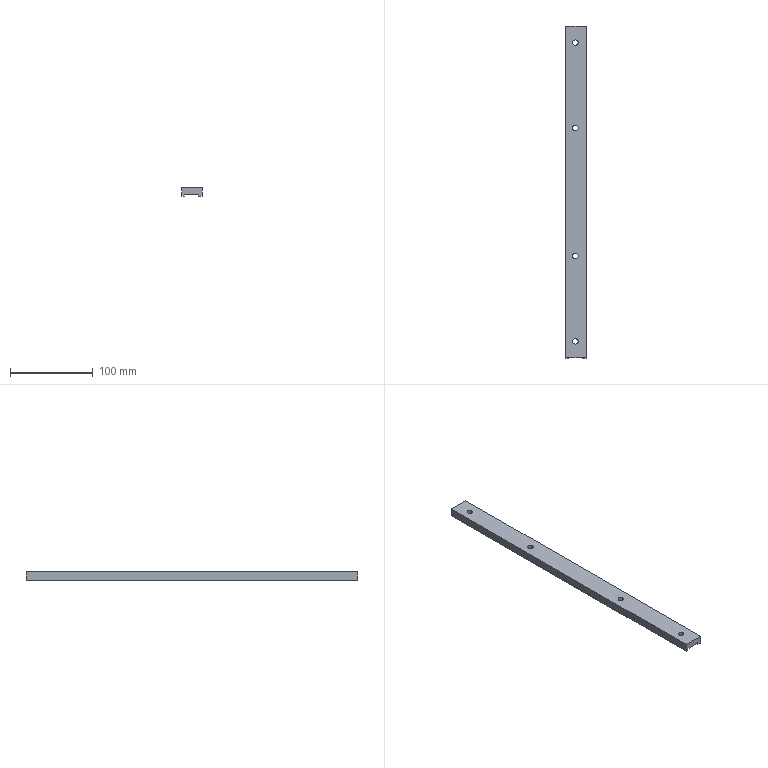Part | SolidWorks | features BaseBody 1 | 1 solid | 26 faces | box 24.5 x 400 x 10 mm | volume 80117 mm3 | plane 10 | cone 8 | cylinder 8 | commonest cylinder face diameters 6.6 x8
STEP:
#1=CARTESIAN_POINT('',(14.8,180.,-4.5));
#2=VERTEX_POINT('',#1);
#3=CARTESIAN_POINT('',(8.2,180.,-4.5));
#4=VERTEX_POINT('',#3);
#5=CARTESIAN_POINT('',(11.5,180.,-4.5));
#6=DIRECTION('',(0.,0.,-1.));
#7=DIRECTION('',(-1.,0.,0.));
#8=AXIS2_PLACEMENT_3D('',#5,#6,#7);
#9=CIRCLE('',#8,3.3);
#10=EDGE_CURVE('',#2,#4,#9,.T.);
#11=ORIENTED_EDGE('',*,*,#10,.F.);
#12=CARTESIAN_POINT('',(17.9,180.,-7.6));
#13=VERTEX_POINT('',#12);
#14=CARTESIAN_POINT('',(17.9,180.,-7.6));
#15=DIRECTION('',(0.7071,0.,-0.7071));
#16=VECTOR('',#15,1000.);
#17=LINE('',#14,#16);
#18=EDGE_CURVE('',#2,#13,#17,.T.);
#19=ORIENTED_EDGE('',*,*,#18,.T.);
#20=CARTESIAN_POINT('',(5.1,180.,-7.6));
#21=VERTEX_POINT('',#20);
#22=CARTESIAN_POINT('',(11.5,180.,-7.6));
#23=DIRECTION('',(0.,0.,-1.));
#24=DIRECTION('',(-1.,0.,0.));
#25=AXIS2_PLACEMENT_3D('',#22,#23,#24);
#26=CIRCLE('',#25,6.4);
#27=EDGE_CURVE('',#13,#21,#26,.T.);
#28=ORIENTED_EDGE('',*,*,#27,.T.);
#29=CARTESIAN_POINT('',(5.1,180.,-7.6));
#30=DIRECTION('',(-0.7071,0.,-0.7071));
#31=VECTOR('',#30,1000.);
#32=LINE('',#29,#31);
#33=EDGE_CURVE('',#4,#21,#32,.T.);
#34=ORIENTED_EDGE('',*,*,#33,.F.);
#35=EDGE_LOOP('',(#11,#19,#28,#34));
#36=FACE_OUTER_BOUND('',#35,.T.);
#37=CARTESIAN_POINT('',(11.5,180.,-7.6));
#38=DIRECTION('',(0.,0.,-1.));
#39=DIRECTION('',(-1.,0.,0.));
#40=AXIS2_PLACEMENT_3D('',#37,#38,#39);
#41=CONICAL_SURFACE('',#40,6.4,0.7854);
#42=ADVANCED_FACE('',(#36),#41,.F.);
#43=CARTESIAN_POINT('',(14.8,180.,0.));
#44=VERTEX_POINT('',#43);
#45=CARTESIAN_POINT('',(8.2,180.,0.));
#46=VERTEX_POINT('',#45);
#47=CARTESIAN_POINT('',(11.5,180.,0.));
#48=DIRECTION('',(0.,0.,-1.));
#49=DIRECTION('',(-1.,0.,0.));
#50=AXIS2_PLACEMENT_3D('',#47,#48,#49);
#51=CIRCLE('',#50,3.3);
#52=EDGE_CURVE('',#44,#46,#51,.T.);
#53=ORIENTED_EDGE('',*,*,#52,.F.);
#54=CARTESIAN_POINT('',(14.8,180.,-7.6));
#55=DIRECTION('',(0.,0.,-1.));
#56=VECTOR('',#55,1000.);
#57=LINE('',#54,#56);
#58=EDGE_CURVE('',#44,#2,#57,.T.);
#59=ORIENTED_EDGE('',*,*,#58,.T.);
#60=ORIENTED_EDGE('',*,*,#10,.T.);
#61=CARTESIAN_POINT('',(8.2,180.,-7.6));
#62=DIRECTION('',(0.,0.,-1.));
#63=VECTOR('',#62,1000.);
#64=LINE('',#61,#63);
#65=EDGE_CURVE('',#46,#4,#64,.T.);
#66=ORIENTED_EDGE('',*,*,#65,.F.);
#67=EDGE_LOOP('',(#53,#59,#60,#66));
#68=FACE_OUTER_BOUND('',#67,.T.);
#69=CARTESIAN_POINT('',(11.5,180.,-7.6));
#70=DIRECTION('',(0.,0.,-1.));
#71=DIRECTION('',(-1.,0.,0.));
#72=AXIS2_PLACEMENT_3D('',#69,#70,#71);
#73=CYLINDRICAL_SURFACE('',#72,3.3);
#74=ADVANCED_FACE('',(#68),#73,.F.);
#75=CARTESIAN_POINT('',(14.8,77.,-4.5));
#76=VERTEX_POINT('',#75);
#77=CARTESIAN_POINT('',(8.2,77.,-4.5));
#78=VERTEX_POINT('',#77);
#79=CARTESIAN_POINT('',(11.5,77.,-4.5));
#80=DIRECTION('',(0.,0.,-1.));
#81=DIRECTION('',(-1.,0.,0.));
#82=AXIS2_PLACEMENT_3D('',#79,#80,#81);
#83=CIRCLE('',#82,3.3);
#84=EDGE_CURVE('',#76,#78,#83,.T.);
#85=ORIENTED_EDGE('',*,*,#84,.F.);
#86=CARTESIAN_POINT('',(17.9,77.,-7.6));
#87=VERTEX_POINT('',#86);
#88=CARTESIAN_POINT('',(17.9,77.,-7.6));
#89=DIRECTION('',(0.7071,0.,-0.7071));
#90=VECTOR('',#89,1000.);
#91=LINE('',#88,#90);
#92=EDGE_CURVE('',#76,#87,#91,.T.);
#93=ORIENTED_EDGE('',*,*,#92,.T.);
#94=CARTESIAN_POINT('',(5.1,77.,-7.6));
#95=VERTEX_POINT('',#94);
#96=CARTESIAN_POINT('',(11.5,77.,-7.6));
#97=DIRECTION('',(0.,0.,-1.));
#98=DIRECTION('',(-1.,0.,0.));
#99=AXIS2_PLACEMENT_3D('',#96,#97,#98);
#100=CIRCLE('',#99,6.4);
#101=EDGE_CURVE('',#87,#95,#100,.T.);
#102=ORIENTED_EDGE('',*,*,#101,.T.);
#103=CARTESIAN_POINT('',(5.1,77.,-7.6));
#104=DIRECTION('',(-0.7071,0.,-0.7071));
#105=VECTOR('',#104,1000.);
#106=LINE('',#103,#105);
#107=EDGE_CURVE('',#78,#95,#106,.T.);
#108=ORIENTED_EDGE('',*,*,#107,.F.);
#109=EDGE_LOOP('',(#85,#93,#102,#108));
#110=FACE_OUTER_BOUND('',#109,.T.);
#111=CARTESIAN_POINT('',(11.5,77.,-7.6));
#112=DIRECTION('',(0.,0.,-1.));
#113=DIRECTION('',(-1.,0.,0.));
#114=AXIS2_PLACEMENT_3D('',#111,#112,#113);
#115=CONICAL_SURFACE('',#114,6.4,0.7854);
#116=ADVANCED_FACE('',(#110),#115,.F.);
#117=CARTESIAN_POINT('',(14.8,77.,0.));
#118=VERTEX_POINT('',#117);
#119=CARTESIAN_POINT('',(8.2,77.,0.));
#120=VERTEX_POINT('',#119);
#121=CARTESIAN_POINT('',(11.5,77.,0.));
#122=DIRECTION('',(0.,0.,-1.));
#123=DIRECTION('',(-1.,0.,0.));
#124=AXIS2_PLACEMENT_3D('',#121,#122,#123);
#125=CIRCLE('',#124,3.3);
#126=EDGE_CURVE('',#118,#120,#125,.T.);
#127=ORIENTED_EDGE('',*,*,#126,.F.);
#128=CARTESIAN_POINT('',(14.8,77.,-7.6));
#129=DIRECTION('',(0.,0.,-1.));
#130=VECTOR('',#129,1000.);
#131=LINE('',#128,#130);
#132=EDGE_CURVE('',#118,#76,#131,.T.);
#133=ORIENTED_EDGE('',*,*,#132,.T.);
#134=ORIENTED_EDGE('',*,*,#84,.T.);
#135=CARTESIAN_POINT('',(8.2,77.,-7.6));
#136=DIRECTION('',(0.,0.,-1.));
#137=VECTOR('',#136,1000.);
#138=LINE('',#135,#137);
#139=EDGE_CURVE('',#120,#78,#138,.T.);
#140=ORIENTED_EDGE('',*,*,#139,.F.);
#141=EDGE_LOOP('',(#127,#133,#134,#140));
#142=FACE_OUTER_BOUND('',#141,.T.);
#143=CARTESIAN_POINT('',(11.5,77.,-7.6));
#144=DIRECTION('',(0.,0.,-1.));
#145=DIRECTION('',(-1.,0.,0.));
#146=AXIS2_PLACEMENT_3D('',#143,#144,#145);
#147=CYLINDRICAL_SURFACE('',#146,3.3);
#148=ADVANCED_FACE('',(#142),#147,.F.);
#149=CARTESIAN_POINT('',(14.8,-77.,-4.5));
#150=VERTEX_POINT('',#149);
#151=CARTESIAN_POINT('',(8.2,-77.,-4.5));
#152=VERTEX_POINT('',#151);
#153=CARTESIAN_POINT('',(11.5,-77.,-4.5));
#154=DIRECTION('',(0.,0.,-1.));
#155=DIRECTION('',(-1.,0.,0.));
#156=AXIS2_PLACEMENT_3D('',#153,#154,#155);
#157=CIRCLE('',#156,3.3);
#158=EDGE_CURVE('',#150,#152,#157,.T.);
#159=ORIENTED_EDGE('',*,*,#158,.F.);
#160=CARTESIAN_POINT('',(17.9,-77.,-7.6));
#161=VERTEX_POINT('',#160);
#162=CARTESIAN_POINT('',(17.9,-77.,-7.6));
#163=DIRECTION('',(0.7071,0.,-0.7071));
#164=VECTOR('',#163,1000.);
#165=LINE('',#162,#164);
#166=EDGE_CURVE('',#150,#161,#165,.T.);
#167=ORIENTED_EDGE('',*,*,#166,.T.);
#168=CARTESIAN_POINT('',(5.1,-77.,-7.6));
#169=VERTEX_POINT('',#168);
#170=CARTESIAN_POINT('',(11.5,-77.,-7.6));
#171=DIRECTION('',(0.,0.,-1.));
#172=DIRECTION('',(-1.,0.,0.));
#173=AXIS2_PLACEMENT_3D('',#170,#171,#172);
#174=CIRCLE('',#173,6.4);
#175=EDGE_CURVE('',#161,#169,#174,.T.);
#176=ORIENTED_EDGE('',*,*,#175,.T.);
#177=CARTESIAN_POINT('',(5.1,-77.,-7.6));
#178=DIRECTION('',(-0.7071,0.,-0.7071));
#179=VECTOR('',#178,1000.);
#180=LINE('',#177,#179);
#181=EDGE_CURVE('',#152,#169,#180,.T.);
#182=ORIENTED_EDGE('',*,*,#181,.F.);
#183=EDGE_LOOP('',(#159,#167,#176,#182));
#184=FACE_OUTER_BOUND('',#183,.T.);
#185=CARTESIAN_POINT('',(11.5,-77.,-7.6));
#186=DIRECTION('',(0.,0.,-1.));
#187=DIRECTION('',(-1.,0.,0.));
#188=AXIS2_PLACEMENT_3D('',#185,#186,#187);
#189=CONICAL_SURFACE('',#188,6.4,0.7854);
#190=ADVANCED_FACE('',(#184),#189,.F.);
#191=CARTESIAN_POINT('',(14.8,-77.,0.));
#192=VERTEX_POINT('',#191);
#193=CARTESIAN_POINT('',(8.2,-77.,0.));
#194=VERTEX_POINT('',#193);
#195=CARTESIAN_POINT('',(11.5,-77.,0.));
#196=DIRECTION('',(0.,0.,-1.));
#197=DIRECTION('',(-1.,0.,0.));
#198=AXIS2_PLACEMENT_3D('',#195,#196,#197);
#199=CIRCLE('',#198,3.3);
#200=EDGE_CURVE('',#192,#194,#199,.T.);
#201=ORIENTED_EDGE('',*,*,#200,.F.);
#202=CARTESIAN_POINT('',(14.8,-77.,-7.6));
#203=DIRECTION('',(0.,0.,-1.));
#204=VECTOR('',#203,1000.);
#205=LINE('',#202,#204);
#206=EDGE_CURVE('',#192,#150,#205,.T.);
#207=ORIENTED_EDGE('',*,*,#206,.T.);
#208=ORIENTED_EDGE('',*,*,#158,.T.);
#209=CARTESIAN_POINT('',(8.2,-77.,-7.6));
#210=DIRECTION('',(0.,0.,-1.));
#211=VECTOR('',#210,1000.);
#212=LINE('',#209,#211);
#213=EDGE_CURVE('',#194,#152,#212,.T.);
#214=ORIENTED_EDGE('',*,*,#213,.F.);
#215=EDGE_LOOP('',(#201,#207,#208,#214));
#216=FACE_OUTER_BOUND('',#215,.T.);
#217=CARTESIAN_POINT('',(11.5,-77.,-7.6));
#218=DIRECTION('',(0.,0.,-1.));
#219=DIRECTION('',(-1.,0.,0.));
#220=AXIS2_PLACEMENT_3D('',#217,#218,#219);
#221=CYLINDRICAL_SURFACE('',#220,3.3);
#222=ADVANCED_FACE('',(#216),#221,.F.);
#223=CARTESIAN_POINT('',(14.8,-180.,-4.5));
#224=VERTEX_POINT('',#223);
#225=CARTESIAN_POINT('',(8.2,-180.,-4.5));
#226=VERTEX_POINT('',#225);
#227=CARTESIAN_POINT('',(11.5,-180.,-4.5));
#228=DIRECTION('',(0.,0.,-1.));
#229=DIRECTION('',(-1.,0.,0.));
#230=AXIS2_PLACEMENT_3D('',#227,#228,#229);
#231=CIRCLE('',#230,3.3);
#232=EDGE_CURVE('',#224,#226,#231,.T.);
#233=ORIENTED_EDGE('',*,*,#232,.F.);
#234=CARTESIAN_POINT('',(17.9,-180.,-7.6));
#235=VERTEX_POINT('',#234);
#236=CARTESIAN_POINT('',(17.9,-180.,-7.6));
#237=DIRECTION('',(0.7071,0.,-0.7071));
#238=VECTOR('',#237,1000.);
#239=LINE('',#236,#238);
#240=EDGE_CURVE('',#224,#235,#239,.T.);
#241=ORIENTED_EDGE('',*,*,#240,.T.);
#242=CARTESIAN_POINT('',(5.1,-180.,-7.6));
#243=VERTEX_POINT('',#242);
#244=CARTESIAN_POINT('',(11.5,-180.,-7.6));
#245=DIRECTION('',(0.,0.,-1.));
#246=DIRECTION('',(-1.,0.,0.));
#247=AXIS2_PLACEMENT_3D('',#244,#245,#246);
#248=CIRCLE('',#247,6.4);
#249=EDGE_CURVE('',#235,#243,#248,.T.);
#250=ORIENTED_EDGE('',*,*,#249,.T.);
#251=CARTESIAN_POINT('',(5.1,-180.,-7.6));
#252=DIRECTION('',(-0.7071,0.,-0.7071));
#253=VECTOR('',#252,1000.);
#254=LINE('',#251,#253);
#255=EDGE_CURVE('',#226,#243,#254,.T.);
#256=ORIENTED_EDGE('',*,*,#255,.F.);
#257=EDGE_LOOP('',(#233,#241,#250,#256));
#258=FACE_OUTER_BOUND('',#257,.T.);
#259=CARTESIAN_POINT('',(11.5,-180.,-7.6));
#260=DIRECTION('',(0.,0.,-1.));
#261=DIRECTION('',(-1.,0.,0.));
#262=AXIS2_PLACEMENT_3D('',#259,#260,#261);
#263=CONICAL_SURFACE('',#262,6.4,0.7854);
#264=ADVANCED_FACE('',(#258),#263,.F.);
#265=CARTESIAN_POINT('',(14.8,-180.,0.));
#266=VERTEX_POINT('',#265);
#267=CARTESIAN_POINT('',(8.2,-180.,0.));
#268=VERTEX_POINT('',#267);
#269=CARTESIAN_POINT('',(11.5,-180.,0.));
#270=DIRECTION('',(0.,0.,-1.));
#271=DIRECTION('',(-1.,0.,0.));
#272=AXIS2_PLACEMENT_3D('',#269,#270,#271);
#273=CIRCLE('',#272,3.3);
#274=EDGE_CURVE('',#266,#268,#273,.T.);
#275=ORIENTED_EDGE('',*,*,#274,.F.);
#276=CARTESIAN_POINT('',(14.8,-180.,-7.6));
#277=DIRECTION('',(0.,0.,-1.));
#278=VECTOR('',#277,1000.);
#279=LINE('',#276,#278);
#280=EDGE_CURVE('',#266,#224,#279,.T.);
#281=ORIENTED_EDGE('',*,*,#280,.T.);
#282=ORIENTED_EDGE('',*,*,#232,.T.);
#283=CARTESIAN_POINT('',(8.2,-180.,-7.6));
#284=DIRECTION('',(0.,0.,-1.));
#285=VECTOR('',#284,1000.);
#286=LINE('',#283,#285);
#287=EDGE_CURVE('',#268,#226,#286,.T.);
#288=ORIENTED_EDGE('',*,*,#287,.F.);
#289=EDGE_LOOP('',(#275,#281,#282,#288));
#290=FACE_OUTER_BOUND('',#289,.T.);
#291=CARTESIAN_POINT('',(11.5,-180.,-7.6));
#292=DIRECTION('',(0.,0.,-1.));
#293=DIRECTION('',(-1.,0.,0.));
#294=AXIS2_PLACEMENT_3D('',#291,#292,#293);
#295=CYLINDRICAL_SURFACE('',#294,3.3);
#296=ADVANCED_FACE('',(#290),#295,.F.);
#297=CARTESIAN_POINT('',(0.,-200.,0.));
#298=VERTEX_POINT('',#297);
#299=CARTESIAN_POINT('',(24.5,-200.,0.));
#300=VERTEX_POINT('',#299);
#301=CARTESIAN_POINT('',(24.5,-200.,0.));
#302=DIRECTION('',(1.,0.,0.));
#303=VECTOR('',#302,1000.);
#304=LINE('',#301,#303);
#305=EDGE_CURVE('',#298,#300,#304,.T.);
#306=ORIENTED_EDGE('',*,*,#305,.F.);
#307=CARTESIAN_POINT('',(0.,-200.,-10.));
#308=VERTEX_POINT('',#307);
#309=CARTESIAN_POINT('',(0.,-200.,0.));
#310=DIRECTION('',(0.,0.,1.));
#311=VECTOR('',#310,1000.);
#312=LINE('',#309,#311);
#313=EDGE_CURVE('',#308,#298,#312,.T.);
#314=ORIENTED_EDGE('',*,*,#313,.F.);
#315=CARTESIAN_POINT('',(3.,-200.,-10.));
#316=VERTEX_POINT('',#315);
#317=CARTESIAN_POINT('',(0.,-200.,-10.));
#318=DIRECTION('',(-1.,0.,0.));
#319=VECTOR('',#318,1000.);
#320=LINE('',#317,#319);
#321=EDGE_CURVE('',#316,#308,#320,.T.);
#322=ORIENTED_EDGE('',*,*,#321,.F.);
#323=CARTESIAN_POINT('',(3.,-200.,-7.6));
#324=VERTEX_POINT('',#323);
#325=CARTESIAN_POINT('',(3.,-200.,-7.6));
#326=DIRECTION('',(0.,0.,-1.));
#327=VECTOR('',#326,1000.);
#328=LINE('',#325,#327);
#329=EDGE_CURVE('',#324,#316,#328,.T.);
#330=ORIENTED_EDGE('',*,*,#329,.F.);
#331=CARTESIAN_POINT('',(20.,-200.,-7.6));
#332=VERTEX_POINT('',#331);
#333=CARTESIAN_POINT('',(3.,-200.,-7.6));
#334=DIRECTION('',(-1.,0.,0.));
#335=VECTOR('',#334,1000.);
#336=LINE('',#333,#335);
#337=EDGE_CURVE('',#332,#324,#336,.T.);
#338=ORIENTED_EDGE('',*,*,#337,.F.);
#339=CARTESIAN_POINT('',(20.,-200.,-10.));
#340=VERTEX_POINT('',#339);
#341=CARTESIAN_POINT('',(20.,-200.,-7.6));
#342=DIRECTION('',(0.,0.,1.));
#343=VECTOR('',#342,1000.);
#344=LINE('',#341,#343);
#345=EDGE_CURVE('',#340,#332,#344,.T.);
#346=ORIENTED_EDGE('',*,*,#345,.F.);
#347=CARTESIAN_POINT('',(24.5,-200.,-10.));
#348=VERTEX_POINT('',#347);
#349=CARTESIAN_POINT('',(20.,-200.,-10.));
#350=DIRECTION('',(-1.,0.,0.));
#351=VECTOR('',#350,1000.);
#352=LINE('',#349,#351);
#353=EDGE_CURVE('',#348,#340,#352,.T.);
#354=ORIENTED_EDGE('',*,*,#353,.F.);
#355=CARTESIAN_POINT('',(24.5,-200.,-10.));
#356=DIRECTION('',(0.,0.,-1.));
#357=VECTOR('',#356,1000.);
#358=LINE('',#355,#357);
#359=EDGE_CURVE('',#300,#348,#358,.T.);
#360=ORIENTED_EDGE('',*,*,#359,.F.);
#361=EDGE_LOOP('',(#306,#314,#322,#330,#338,#346,#354,#360));
#362=FACE_OUTER_BOUND('',#361,.T.);
#363=CARTESIAN_POINT('',(0.,-200.,0.));
#364=DIRECTION('',(0.,-1.,0.));
#365=DIRECTION('',(0.,0.,-1.));
#366=AXIS2_PLACEMENT_3D('',#363,#364,#365);
#367=PLANE('',#366);
#368=ADVANCED_FACE('',(#362),#367,.T.);
#369=CARTESIAN_POINT('',(0.,200.,0.));
#370=VERTEX_POINT('',#369);
#371=CARTESIAN_POINT('',(24.5,200.,0.));
#372=VERTEX_POINT('',#371);
#373=CARTESIAN_POINT('',(24.5,200.,0.));
#374=DIRECTION('',(1.,0.,0.));
#375=VECTOR('',#374,1000.);
#376=LINE('',#373,#375);
#377=EDGE_CURVE('',#370,#372,#376,.T.);
#378=ORIENTED_EDGE('',*,*,#377,.T.);
#379=CARTESIAN_POINT('',(24.5,200.,-10.));
#380=VERTEX_POINT('',#379);
#381=CARTESIAN_POINT('',(24.5,200.,-10.));
#382=DIRECTION('',(0.,0.,-1.));
#383=VECTOR('',#382,1000.);
#384=LINE('',#381,#383);
#385=EDGE_CURVE('',#372,#380,#384,.T.);
#386=ORIENTED_EDGE('',*,*,#385,.T.);
#387=CARTESIAN_POINT('',(20.,200.,-10.));
#388=VERTEX_POINT('',#387);
#389=CARTESIAN_POINT('',(20.,200.,-10.));
#390=DIRECTION('',(-1.,0.,0.));
#391=VECTOR('',#390,1000.);
#392=LINE('',#389,#391);
#393=EDGE_CURVE('',#380,#388,#392,.T.);
#394=ORIENTED_EDGE('',*,*,#393,.T.);
#395=CARTESIAN_POINT('',(20.,200.,-7.6));
#396=VERTEX_POINT('',#395);
#397=CARTESIAN_POINT('',(20.,200.,-7.6));
#398=DIRECTION('',(0.,0.,1.));
#399=VECTOR('',#398,1000.);
#400=LINE('',#397,#399);
#401=EDGE_CURVE('',#388,#396,#400,.T.);
#402=ORIENTED_EDGE('',*,*,#401,.T.);
#403=CARTESIAN_POINT('',(3.,200.,-7.6));
#404=VERTEX_POINT('',#403);
#405=CARTESIAN_POINT('',(3.,200.,-7.6));
#406=DIRECTION('',(-1.,0.,0.));
#407=VECTOR('',#406,1000.);
#408=LINE('',#405,#407);
#409=EDGE_CURVE('',#396,#404,#408,.T.);
#410=ORIENTED_EDGE('',*,*,#409,.T.);
#411=CARTESIAN_POINT('',(3.,200.,-10.));
#412=VERTEX_POINT('',#411);
#413=CARTESIAN_POINT('',(3.,200.,-7.6));
#414=DIRECTION('',(0.,0.,-1.));
#415=VECTOR('',#414,1000.);
#416=LINE('',#413,#415);
#417=EDGE_CURVE('',#404,#412,#416,.T.);
#418=ORIENTED_EDGE('',*,*,#417,.T.);
#419=CARTESIAN_POINT('',(0.,200.,-10.));
#420=VERTEX_POINT('',#419);
#421=CARTESIAN_POINT('',(0.,200.,-10.));
#422=DIRECTION('',(-1.,0.,0.));
#423=VECTOR('',#422,1000.);
#424=LINE('',#421,#423);
#425=EDGE_CURVE('',#412,#420,#424,.T.);
#426=ORIENTED_EDGE('',*,*,#425,.T.);
#427=CARTESIAN_POINT('',(0.,200.,0.));
#428=DIRECTION('',(0.,0.,1.));
#429=VECTOR('',#428,1000.);
#430=LINE('',#427,#429);
#431=EDGE_CURVE('',#420,#370,#430,.T.);
#432=ORIENTED_EDGE('',*,*,#431,.T.);
#433=EDGE_LOOP('',(#378,#386,#394,#402,#410,#418,#426,#432));
#434=FACE_OUTER_BOUND('',#433,.T.);
#435=CARTESIAN_POINT('',(0.,200.,0.));
#436=DIRECTION('',(0.,-1.,0.));
#437=DIRECTION('',(0.,0.,-1.));
#438=AXIS2_PLACEMENT_3D('',#435,#436,#437);
#439=PLANE('',#438);
#440=ADVANCED_FACE('',(#434),#439,.F.);
#441=ORIENTED_EDGE('',*,*,#313,.T.);
#442=CARTESIAN_POINT('',(0.,200.,0.));
#443=DIRECTION('',(0.,-1.,0.));
#444=VECTOR('',#443,1000.);
#445=LINE('',#442,#444);
#446=EDGE_CURVE('',#370,#298,#445,.T.);
#447=ORIENTED_EDGE('',*,*,#446,.F.);
#448=ORIENTED_EDGE('',*,*,#431,.F.);
#449=CARTESIAN_POINT('',(0.,200.,-10.));
#450=DIRECTION('',(0.,-1.,0.));
#451=VECTOR('',#450,1000.);
#452=LINE('',#449,#451);
#453=EDGE_CURVE('',#420,#308,#452,.T.);
#454=ORIENTED_EDGE('',*,*,#453,.T.);
#455=EDGE_LOOP('',(#441,#447,#448,#454));
#456=FACE_OUTER_BOUND('',#455,.T.);
#457=CARTESIAN_POINT('',(0.,200.,0.));
#458=DIRECTION('',(1.,0.,0.));
#459=DIRECTION('',(0.,1.,0.));
#460=AXIS2_PLACEMENT_3D('',#457,#458,#459);
#461=PLANE('',#460);
#462=ADVANCED_FACE('',(#456),#461,.F.);
#463=ORIENTED_EDGE('',*,*,#321,.T.);
#464=ORIENTED_EDGE('',*,*,#453,.F.);
#465=ORIENTED_EDGE('',*,*,#425,.F.);
#466=CARTESIAN_POINT('',(3.,200.,-10.));
#467=DIRECTION('',(0.,-1.,0.));
#468=VECTOR('',#467,1000.);
#469=LINE('',#466,#468);
#470=EDGE_CURVE('',#412,#316,#469,.T.);
#471=ORIENTED_EDGE('',*,*,#470,.T.);
#472=EDGE_LOOP('',(#463,#464,#465,#471));
#473=FACE_OUTER_BOUND('',#472,.T.);
#474=CARTESIAN_POINT('',(0.,200.,-10.));
#475=DIRECTION('',(0.,0.,1.));
#476=DIRECTION('',(1.,0.,0.));
#477=AXIS2_PLACEMENT_3D('',#474,#475,#476);
#478=PLANE('',#477);
#479=ADVANCED_FACE('',(#473),#478,.F.);
#480=ORIENTED_EDGE('',*,*,#329,.T.);
#481=ORIENTED_EDGE('',*,*,#470,.F.);
#482=ORIENTED_EDGE('',*,*,#417,.F.);
#483=CARTESIAN_POINT('',(3.,200.,-7.6));
#484=DIRECTION('',(0.,-1.,0.));
#485=VECTOR('',#484,1000.);
#486=LINE('',#483,#485);
#487=EDGE_CURVE('',#404,#324,#486,.T.);
#488=ORIENTED_EDGE('',*,*,#487,.T.);
#489=EDGE_LOOP('',(#480,#481,#482,#488));
#490=FACE_OUTER_BOUND('',#489,.T.);
#491=CARTESIAN_POINT('',(3.,200.,-7.6));
#492=DIRECTION('',(-1.,0.,0.));
#493=DIRECTION('',(0.,0.,1.));
#494=AXIS2_PLACEMENT_3D('',#491,#492,#493);
#495=PLANE('',#494);
#496=ADVANCED_FACE('',(#490),#495,.F.);
#497=CARTESIAN_POINT('',(11.5,-180.,-7.6));
#498=DIRECTION('',(0.,0.,-1.));
#499=DIRECTION('',(-1.,0.,0.));
#500=AXIS2_PLACEMENT_3D('',#497,#498,#499);
#501=CIRCLE('',#500,6.4);
#502=EDGE_CURVE('',#243,#235,#501,.T.);
#503=ORIENTED_EDGE('',*,*,#502,.F.);
#504=ORIENTED_EDGE('',*,*,#249,.F.);
#505=EDGE_LOOP('',(#503,#504));
#506=FACE_BOUND('',#505,.T.);
#507=CARTESIAN_POINT('',(11.5,-77.,-7.6));
#508=DIRECTION('',(0.,0.,-1.));
#509=DIRECTION('',(-1.,0.,0.));
#510=AXIS2_PLACEMENT_3D('',#507,#508,#509);
#511=CIRCLE('',#510,6.4);
#512=EDGE_CURVE('',#169,#161,#511,.T.);
#513=ORIENTED_EDGE('',*,*,#512,.F.);
#514=ORIENTED_EDGE('',*,*,#175,.F.);
#515=EDGE_LOOP('',(#513,#514));
#516=FACE_BOUND('',#515,.T.);
#517=CARTESIAN_POINT('',(11.5,77.,-7.6));
#518=DIRECTION('',(0.,0.,-1.));
#519=DIRECTION('',(-1.,0.,0.));
#520=AXIS2_PLACEMENT_3D('',#517,#518,#519);
#521=CIRCLE('',#520,6.4);
#522=EDGE_CURVE('',#95,#87,#521,.T.);
#523=ORIENTED_EDGE('',*,*,#522,.F.);
#524=ORIENTED_EDGE('',*,*,#101,.F.);
#525=EDGE_LOOP('',(#523,#524));
#526=FACE_BOUND('',#525,.T.);
#527=CARTESIAN_POINT('',(11.5,180.,-7.6));
#528=DIRECTION('',(0.,0.,-1.));
#529=DIRECTION('',(-1.,0.,0.));
#530=AXIS2_PLACEMENT_3D('',#527,#528,#529);
#531=CIRCLE('',#530,6.4);
#532=EDGE_CURVE('',#21,#13,#531,.T.);
#533=ORIENTED_EDGE('',*,*,#532,.F.);
#534=ORIENTED_EDGE('',*,*,#27,.F.);
#535=EDGE_LOOP('',(#533,#534));
#536=FACE_BOUND('',#535,.T.);
#537=ORIENTED_EDGE('',*,*,#337,.T.);
#538=ORIENTED_EDGE('',*,*,#487,.F.);
#539=ORIENTED_EDGE('',*,*,#409,.F.);
#540=CARTESIAN_POINT('',(20.,200.,-7.6));
#541=DIRECTION('',(0.,-1.,0.));
#542=VECTOR('',#541,1000.);
#543=LINE('',#540,#542);
#544=EDGE_CURVE('',#396,#332,#543,.T.);
#545=ORIENTED_EDGE('',*,*,#544,.T.);
#546=EDGE_LOOP('',(#537,#538,#539,#545));
#547=FACE_OUTER_BOUND('',#546,.T.);
#548=CARTESIAN_POINT('',(3.,200.,-7.6));
#549=DIRECTION('',(0.,0.,1.));
#550=DIRECTION('',(1.,0.,0.));
#551=AXIS2_PLACEMENT_3D('',#548,#549,#550);
#552=PLANE('',#551);
#553=ADVANCED_FACE('',(#506,#516,#526,#536,#547),#552,.F.);
#554=ORIENTED_EDGE('',*,*,#345,.T.);
#555=ORIENTED_EDGE('',*,*,#544,.F.);
#556=ORIENTED_EDGE('',*,*,#401,.F.);
#557=CARTESIAN_POINT('',(20.,200.,-10.));
#558=DIRECTION('',(0.,-1.,0.));
#559=VECTOR('',#558,1000.);
#560=LINE('',#557,#559);
#561=EDGE_CURVE('',#388,#340,#560,.T.);
#562=ORIENTED_EDGE('',*,*,#561,.T.);
#563=EDGE_LOOP('',(#554,#555,#556,#562));
#564=FACE_OUTER_BOUND('',#563,.T.);
#565=CARTESIAN_POINT('',(20.,200.,-7.6));
#566=DIRECTION('',(1.,0.,0.));
#567=DIRECTION('',(0.,1.,0.));
#568=AXIS2_PLACEMENT_3D('',#565,#566,#567);
#569=PLANE('',#568);
#570=ADVANCED_FACE('',(#564),#569,.F.);
#571=ORIENTED_EDGE('',*,*,#353,.T.);
#572=ORIENTED_EDGE('',*,*,#561,.F.);
#573=ORIENTED_EDGE('',*,*,#393,.F.);
#574=CARTESIAN_POINT('',(24.5,200.,-10.));
#575=DIRECTION('',(0.,-1.,0.));
#576=VECTOR('',#575,1000.);
#577=LINE('',#574,#576);
#578=EDGE_CURVE('',#380,#348,#577,.T.);
#579=ORIENTED_EDGE('',*,*,#578,.T.);
#580=EDGE_LOOP('',(#571,#572,#573,#579));
#581=FACE_OUTER_BOUND('',#580,.T.);
#582=CARTESIAN_POINT('',(20.,200.,-10.));
#583=DIRECTION('',(0.,0.,1.));
#584=DIRECTION('',(1.,0.,0.));
#585=AXIS2_PLACEMENT_3D('',#582,#583,#584);
#586=PLANE('',#585);
#587=ADVANCED_FACE('',(#581),#586,.F.);
#588=ORIENTED_EDGE('',*,*,#359,.T.);
#589=ORIENTED_EDGE('',*,*,#578,.F.);
#590=ORIENTED_EDGE('',*,*,#385,.F.);
#591=CARTESIAN_POINT('',(24.5,200.,0.));
#592=DIRECTION('',(0.,-1.,0.));
#593=VECTOR('',#592,1000.);
#594=LINE('',#591,#593);
#595=EDGE_CURVE('',#372,#300,#594,.T.);
#596=ORIENTED_EDGE('',*,*,#595,.T.);
#597=EDGE_LOOP('',(#588,#589,#590,#596));
#598=FACE_OUTER_BOUND('',#597,.T.);
#599=CARTESIAN_POINT('',(24.5,200.,-10.));
#600=DIRECTION('',(-1.,0.,0.));
#601=DIRECTION('',(0.,0.,1.));
#602=AXIS2_PLACEMENT_3D('',#599,#600,#601);
#603=PLANE('',#602);
#604=ADVANCED_FACE('',(#598),#603,.F.);
#605=CARTESIAN_POINT('',(11.5,-180.,0.));
#606=DIRECTION('',(0.,0.,-1.));
#607=DIRECTION('',(-1.,0.,0.));
#608=AXIS2_PLACEMENT_3D('',#605,#606,#607);
#609=CIRCLE('',#608,3.3);
#610=EDGE_CURVE('',#268,#266,#609,.T.);
#611=ORIENTED_EDGE('',*,*,#610,.T.);
#612=ORIENTED_EDGE('',*,*,#274,.T.);
#613=EDGE_LOOP('',(#611,#612));
#614=FACE_BOUND('',#613,.T.);
#615=CARTESIAN_POINT('',(11.5,-77.,0.));
#616=DIRECTION('',(0.,0.,-1.));
#617=DIRECTION('',(-1.,0.,0.));
#618=AXIS2_PLACEMENT_3D('',#615,#616,#617);
#619=CIRCLE('',#618,3.3);
#620=EDGE_CURVE('',#194,#192,#619,.T.);
#621=ORIENTED_EDGE('',*,*,#620,.T.);
#622=ORIENTED_EDGE('',*,*,#200,.T.);
#623=EDGE_LOOP('',(#621,#622));
#624=FACE_BOUND('',#623,.T.);
#625=CARTESIAN_POINT('',(11.5,77.,0.));
#626=DIRECTION('',(0.,0.,-1.));
#627=DIRECTION('',(-1.,0.,0.));
#628=AXIS2_PLACEMENT_3D('',#625,#626,#627);
#629=CIRCLE('',#628,3.3);
#630=EDGE_CURVE('',#120,#118,#629,.T.);
#631=ORIENTED_EDGE('',*,*,#630,.T.);
#632=ORIENTED_EDGE('',*,*,#126,.T.);
#633=EDGE_LOOP('',(#631,#632));
#634=FACE_BOUND('',#633,.T.);
#635=CARTESIAN_POINT('',(11.5,180.,0.));
#636=DIRECTION('',(0.,0.,-1.));
#637=DIRECTION('',(-1.,0.,0.));
#638=AXIS2_PLACEMENT_3D('',#635,#636,#637);
#639=CIRCLE('',#638,3.3);
#640=EDGE_CURVE('',#46,#44,#639,.T.);
#641=ORIENTED_EDGE('',*,*,#640,.T.);
#642=ORIENTED_EDGE('',*,*,#52,.T.);
#643=EDGE_LOOP('',(#641,#642));
#644=FACE_BOUND('',#643,.T.);
#645=ORIENTED_EDGE('',*,*,#305,.T.);
#646=ORIENTED_EDGE('',*,*,#595,.F.);
#647=ORIENTED_EDGE('',*,*,#377,.F.);
#648=ORIENTED_EDGE('',*,*,#446,.T.);
#649=EDGE_LOOP('',(#645,#646,#647,#648));
#650=FACE_OUTER_BOUND('',#649,.T.);
#651=CARTESIAN_POINT('',(24.5,200.,0.));
#652=DIRECTION('',(0.,0.,-1.));
#653=DIRECTION('',(-1.,0.,0.));
#654=AXIS2_PLACEMENT_3D('',#651,#652,#653);
#655=PLANE('',#654);
#656=ADVANCED_FACE('',(#614,#624,#634,#644,#650),#655,.F.);
#657=ORIENTED_EDGE('',*,*,#280,.F.);
#658=ORIENTED_EDGE('',*,*,#610,.F.);
#659=ORIENTED_EDGE('',*,*,#287,.T.);
#660=CARTESIAN_POINT('',(11.5,-180.,-4.5));
#661=DIRECTION('',(0.,0.,-1.));
#662=DIRECTION('',(-1.,0.,0.));
#663=AXIS2_PLACEMENT_3D('',#660,#661,#662);
#664=CIRCLE('',#663,3.3);
#665=EDGE_CURVE('',#226,#224,#664,.T.);
#666=ORIENTED_EDGE('',*,*,#665,.T.);
#667=EDGE_LOOP('',(#657,#658,#659,#666));
#668=FACE_OUTER_BOUND('',#667,.T.);
#669=CARTESIAN_POINT('',(11.5,-180.,-7.6));
#670=DIRECTION('',(0.,0.,-1.));
#671=DIRECTION('',(-1.,0.,0.));
#672=AXIS2_PLACEMENT_3D('',#669,#670,#671);
#673=CYLINDRICAL_SURFACE('',#672,3.3);
#674=ADVANCED_FACE('',(#668),#673,.F.);
#675=ORIENTED_EDGE('',*,*,#240,.F.);
#676=ORIENTED_EDGE('',*,*,#665,.F.);
#677=ORIENTED_EDGE('',*,*,#255,.T.);
#678=ORIENTED_EDGE('',*,*,#502,.T.);
#679=EDGE_LOOP('',(#675,#676,#677,#678));
#680=FACE_OUTER_BOUND('',#679,.T.);
#681=CARTESIAN_POINT('',(11.5,-180.,-7.6));
#682=DIRECTION('',(0.,0.,-1.));
#683=DIRECTION('',(-1.,0.,0.));
#684=AXIS2_PLACEMENT_3D('',#681,#682,#683);
#685=CONICAL_SURFACE('',#684,6.4,0.7854);
#686=ADVANCED_FACE('',(#680),#685,.F.);
#687=ORIENTED_EDGE('',*,*,#206,.F.);
#688=ORIENTED_EDGE('',*,*,#620,.F.);
#689=ORIENTED_EDGE('',*,*,#213,.T.);
#690=CARTESIAN_POINT('',(11.5,-77.,-4.5));
#691=DIRECTION('',(0.,0.,-1.));
#692=DIRECTION('',(-1.,0.,0.));
#693=AXIS2_PLACEMENT_3D('',#690,#691,#692);
#694=CIRCLE('',#693,3.3);
#695=EDGE_CURVE('',#152,#150,#694,.T.);
#696=ORIENTED_EDGE('',*,*,#695,.T.);
#697=EDGE_LOOP('',(#687,#688,#689,#696));
#698=FACE_OUTER_BOUND('',#697,.T.);
#699=CARTESIAN_POINT('',(11.5,-77.,-7.6));
#700=DIRECTION('',(0.,0.,-1.));
#701=DIRECTION('',(-1.,0.,0.));
#702=AXIS2_PLACEMENT_3D('',#699,#700,#701);
#703=CYLINDRICAL_SURFACE('',#702,3.3);
#704=ADVANCED_FACE('',(#698),#703,.F.);
#705=ORIENTED_EDGE('',*,*,#166,.F.);
#706=ORIENTED_EDGE('',*,*,#695,.F.);
#707=ORIENTED_EDGE('',*,*,#181,.T.);
#708=ORIENTED_EDGE('',*,*,#512,.T.);
#709=EDGE_LOOP('',(#705,#706,#707,#708));
#710=FACE_OUTER_BOUND('',#709,.T.);
#711=CARTESIAN_POINT('',(11.5,-77.,-7.6));
#712=DIRECTION('',(0.,0.,-1.));
#713=DIRECTION('',(-1.,0.,0.));
#714=AXIS2_PLACEMENT_3D('',#711,#712,#713);
#715=CONICAL_SURFACE('',#714,6.4,0.7854);
#716=ADVANCED_FACE('',(#710),#715,.F.);
#717=ORIENTED_EDGE('',*,*,#132,.F.);
#718=ORIENTED_EDGE('',*,*,#630,.F.);
#719=ORIENTED_EDGE('',*,*,#139,.T.);
#720=CARTESIAN_POINT('',(11.5,77.,-4.5));
#721=DIRECTION('',(0.,0.,-1.));
#722=DIRECTION('',(-1.,0.,0.));
#723=AXIS2_PLACEMENT_3D('',#720,#721,#722);
#724=CIRCLE('',#723,3.3);
#725=EDGE_CURVE('',#78,#76,#724,.T.);
#726=ORIENTED_EDGE('',*,*,#725,.T.);
#727=EDGE_LOOP('',(#717,#718,#719,#726));
#728=FACE_OUTER_BOUND('',#727,.T.);
#729=CARTESIAN_POINT('',(11.5,77.,-7.6));
#730=DIRECTION('',(0.,0.,-1.));
#731=DIRECTION('',(-1.,0.,0.));
#732=AXIS2_PLACEMENT_3D('',#729,#730,#731);
#733=CYLINDRICAL_SURFACE('',#732,3.3);
#734=ADVANCED_FACE('',(#728),#733,.F.);
#735=ORIENTED_EDGE('',*,*,#92,.F.);
#736=ORIENTED_EDGE('',*,*,#725,.F.);
#737=ORIENTED_EDGE('',*,*,#107,.T.);
#738=ORIENTED_EDGE('',*,*,#522,.T.);
#739=EDGE_LOOP('',(#735,#736,#737,#738));
#740=FACE_OUTER_BOUND('',#739,.T.);
#741=CARTESIAN_POINT('',(11.5,77.,-7.6));
#742=DIRECTION('',(0.,0.,-1.));
#743=DIRECTION('',(-1.,0.,0.));
#744=AXIS2_PLACEMENT_3D('',#741,#742,#743);
#745=CONICAL_SURFACE('',#744,6.4,0.7854);
#746=ADVANCED_FACE('',(#740),#745,.F.);
#747=ORIENTED_EDGE('',*,*,#58,.F.);
#748=ORIENTED_EDGE('',*,*,#640,.F.);
#749=ORIENTED_EDGE('',*,*,#65,.T.);
#750=CARTESIAN_POINT('',(11.5,180.,-4.5));
#751=DIRECTION('',(0.,0.,-1.));
#752=DIRECTION('',(-1.,0.,0.));
#753=AXIS2_PLACEMENT_3D('',#750,#751,#752);
#754=CIRCLE('',#753,3.3);
#755=EDGE_CURVE('',#4,#2,#754,.T.);
#756=ORIENTED_EDGE('',*,*,#755,.T.);
#757=EDGE_LOOP('',(#747,#748,#749,#756));
#758=FACE_OUTER_BOUND('',#757,.T.);
#759=CARTESIAN_POINT('',(11.5,180.,-7.6));
#760=DIRECTION('',(0.,0.,-1.));
#761=DIRECTION('',(-1.,0.,0.));
#762=AXIS2_PLACEMENT_3D('',#759,#760,#761);
#763=CYLINDRICAL_SURFACE('',#762,3.3);
#764=ADVANCED_FACE('',(#758),#763,.F.);
#765=ORIENTED_EDGE('',*,*,#18,.F.);
#766=ORIENTED_EDGE('',*,*,#755,.F.);
#767=ORIENTED_EDGE('',*,*,#33,.T.);
#768=ORIENTED_EDGE('',*,*,#532,.T.);
#769=EDGE_LOOP('',(#765,#766,#767,#768));
#770=FACE_OUTER_BOUND('',#769,.T.);
#771=CARTESIAN_POINT('',(11.5,180.,-7.6));
#772=DIRECTION('',(0.,0.,-1.));
#773=DIRECTION('',(-1.,0.,0.));
#774=AXIS2_PLACEMENT_3D('',#771,#772,#773);
#775=CONICAL_SURFACE('',#774,6.4,0.7854);
#776=ADVANCED_FACE('',(#770),#775,.F.);
#777=CLOSED_SHELL('',(#42,#74,#116,#148,#190,#222,#264,#296,#368,#440,#462,#479,#496,#553,#570,#587,#604,#656,#674,#686,#704,#716,#734,#746,#764,#776));
#778=MANIFOLD_SOLID_BREP('',#777);
#779=CARTESIAN_POINT('',(0.,0.,0.));
#780=DIRECTION('',(0.,0.,1.));
#781=DIRECTION('',(1.,0.,0.));
#782=AXIS2_PLACEMENT_3D('',#779,#780,#781);
#783=(LENGTH_UNIT()NAMED_UNIT(*)SI_UNIT(.MILLI.,.METRE.));
#784=UNCERTAINTY_MEASURE_WITH_UNIT(LENGTH_MEASURE(0.00001),#783,'','');
#785=(NAMED_UNIT(*)PLANE_ANGLE_UNIT()SI_UNIT($,.RADIAN.));
#786=(NAMED_UNIT(*)SI_UNIT($,.STERADIAN.)SOLID_ANGLE_UNIT());
#787=(GEOMETRIC_REPRESENTATION_CONTEXT(3)GLOBAL_UNCERTAINTY_ASSIGNED_CONTEXT((#784))GLOBAL_UNIT_ASSIGNED_CONTEXT((#783,#785,#786))REPRESENTATION_CONTEXT('',''));
#788=ADVANCED_BREP_SHAPE_REPRESENTATION('',(#778,#782),#787);